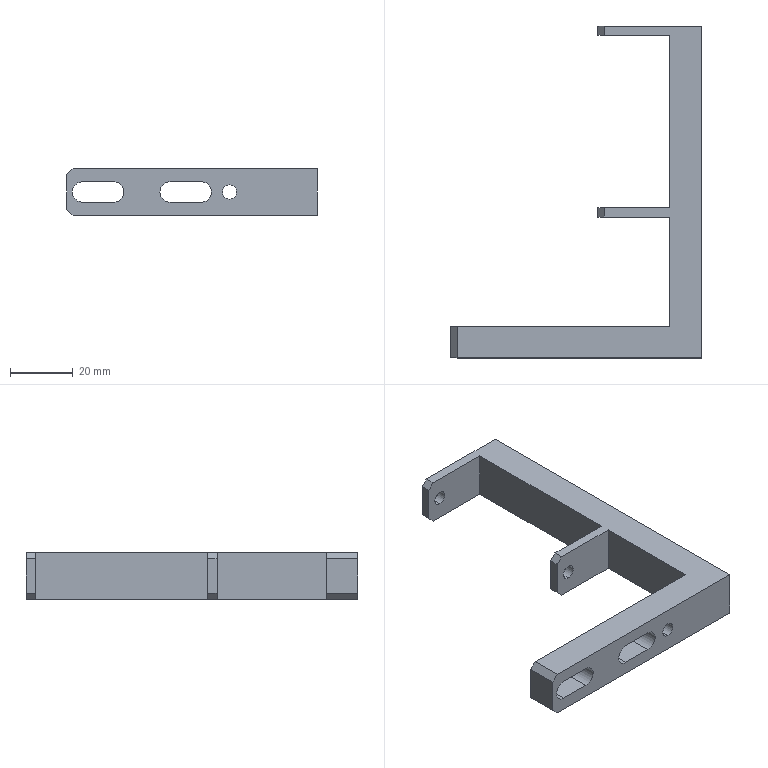Part | STEP file | Rotor photoelectric sensor bracket | 1 solid | 36 faces | box 80 x 106 x 15 mm | volume 26188 mm3 | plane 24 | cylinder 12 | commonest cylinder face diameters 4.5 x6 6.5 x6